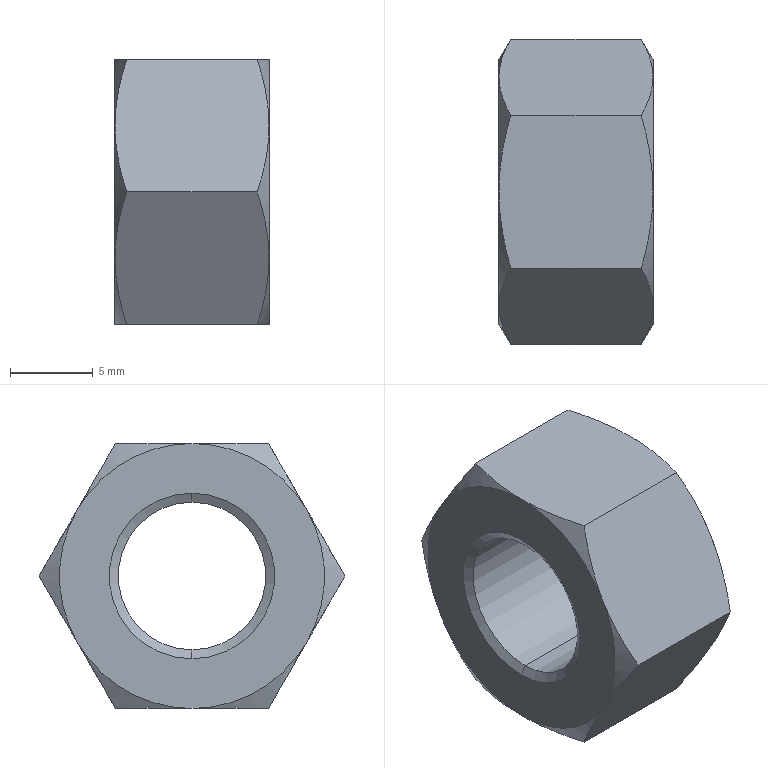Part | SolidWorks | features BaseBody 1 | 1 solid | 26 faces | box 9.3 x 18.475 x 16 mm | volume 1467 mm3 | cone 16 | plane 8 | cylinder 2 | commonest cylinder face diameters 8.917 x2
STEP:
#1=CARTESIAN_POINT('',(0.3125,0.,4.459));
#2=VERTEX_POINT('',#1);
#3=CARTESIAN_POINT('',(0.3125,0.,-4.459));
#4=VERTEX_POINT('',#3);
#5=CARTESIAN_POINT('',(0.3125,0.,0.));
#6=DIRECTION('',(1.,0.,0.));
#7=DIRECTION('',(0.,0.,-1.));
#8=AXIS2_PLACEMENT_3D('',#5,#6,#7);
#9=CIRCLE('',#8,4.459);
#10=EDGE_CURVE('',#2,#4,#9,.T.);
#11=ORIENTED_EDGE('',*,*,#10,.F.);
#12=CARTESIAN_POINT('',(8.987,0.,4.459));
#13=VERTEX_POINT('',#12);
#14=CARTESIAN_POINT('',(-16.85,0.,4.459));
#15=DIRECTION('',(1.,0.,0.));
#16=VECTOR('',#15,1000.);
#17=LINE('',#14,#16);
#18=EDGE_CURVE('',#2,#13,#17,.T.);
#19=ORIENTED_EDGE('',*,*,#18,.T.);
#20=CARTESIAN_POINT('',(8.987,0.,-4.459));
#21=VERTEX_POINT('',#20);
#22=CARTESIAN_POINT('',(8.987,0.,0.));
#23=DIRECTION('',(-1.,0.,0.));
#24=DIRECTION('',(0.,0.,-1.));
#25=AXIS2_PLACEMENT_3D('',#22,#23,#24);
#26=CIRCLE('',#25,4.459);
#27=EDGE_CURVE('',#21,#13,#26,.T.);
#28=ORIENTED_EDGE('',*,*,#27,.F.);
#29=CARTESIAN_POINT('',(-16.85,0.,-4.459));
#30=DIRECTION('',(1.,0.,0.));
#31=VECTOR('',#30,1000.);
#32=LINE('',#29,#31);
#33=EDGE_CURVE('',#4,#21,#32,.T.);
#34=ORIENTED_EDGE('',*,*,#33,.F.);
#35=EDGE_LOOP('',(#11,#19,#28,#34));
#36=FACE_OUTER_BOUND('',#35,.T.);
#37=CARTESIAN_POINT('',(-16.85,0.,0.));
#38=DIRECTION('',(1.,0.,0.));
#39=DIRECTION('',(0.,0.,-1.));
#40=AXIS2_PLACEMENT_3D('',#37,#38,#39);
#41=CYLINDRICAL_SURFACE('',#40,4.459);
#42=ADVANCED_FACE('',(#36),#41,.F.);
#43=ORIENTED_EDGE('',*,*,#10,.T.);
#44=CARTESIAN_POINT('',(0.,0.,-5.));
#45=VERTEX_POINT('',#44);
#46=CARTESIAN_POINT('',(0.,0.,-5.));
#47=DIRECTION('',(-0.5,0.,-0.866));
#48=VECTOR('',#47,1000.);
#49=LINE('',#46,#48);
#50=EDGE_CURVE('',#4,#45,#49,.T.);
#51=ORIENTED_EDGE('',*,*,#50,.T.);
#52=CARTESIAN_POINT('',(0.,0.,5.));
#53=VERTEX_POINT('',#52);
#54=CARTESIAN_POINT('',(0.,0.,0.));
#55=DIRECTION('',(1.,0.,0.));
#56=DIRECTION('',(0.,0.,1.));
#57=AXIS2_PLACEMENT_3D('',#54,#55,#56);
#58=CIRCLE('',#57,5.);
#59=EDGE_CURVE('',#53,#45,#58,.T.);
#60=ORIENTED_EDGE('',*,*,#59,.F.);
#61=CARTESIAN_POINT('',(0.,0.,5.));
#62=DIRECTION('',(-0.5,0.,0.866));
#63=VECTOR('',#62,1000.);
#64=LINE('',#61,#63);
#65=EDGE_CURVE('',#2,#53,#64,.T.);
#66=ORIENTED_EDGE('',*,*,#65,.F.);
#67=EDGE_LOOP('',(#43,#51,#60,#66));
#68=FACE_OUTER_BOUND('',#67,.T.);
#69=CARTESIAN_POINT('',(0.,0.,0.));
#70=DIRECTION('',(-1.,0.,0.));
#71=DIRECTION('',(0.,0.,1.));
#72=AXIS2_PLACEMENT_3D('',#69,#70,#71);
#73=CONICAL_SURFACE('',#72,5.,1.047);
#74=ADVANCED_FACE('',(#68),#73,.F.);
#75=ORIENTED_EDGE('',*,*,#27,.T.);
#76=CARTESIAN_POINT('',(9.3,0.,5.));
#77=VERTEX_POINT('',#76);
#78=CARTESIAN_POINT('',(9.3,0.,5.));
#79=DIRECTION('',(0.5,0.,0.866));
#80=VECTOR('',#79,1000.);
#81=LINE('',#78,#80);
#82=EDGE_CURVE('',#13,#77,#81,.T.);
#83=ORIENTED_EDGE('',*,*,#82,.T.);
#84=CARTESIAN_POINT('',(9.3,0.,-5.));
#85=VERTEX_POINT('',#84);
#86=CARTESIAN_POINT('',(9.3,0.,0.));
#87=DIRECTION('',(-1.,0.,0.));
#88=DIRECTION('',(0.,0.,-1.));
#89=AXIS2_PLACEMENT_3D('',#86,#87,#88);
#90=CIRCLE('',#89,5.);
#91=EDGE_CURVE('',#85,#77,#90,.T.);
#92=ORIENTED_EDGE('',*,*,#91,.F.);
#93=CARTESIAN_POINT('',(9.3,0.,-5.));
#94=DIRECTION('',(0.5,0.,-0.866));
#95=VECTOR('',#94,1000.);
#96=LINE('',#93,#95);
#97=EDGE_CURVE('',#21,#85,#96,.T.);
#98=ORIENTED_EDGE('',*,*,#97,.F.);
#99=EDGE_LOOP('',(#75,#83,#92,#98));
#100=FACE_OUTER_BOUND('',#99,.T.);
#101=CARTESIAN_POINT('',(9.3,0.,0.));
#102=DIRECTION('',(1.,0.,0.));
#103=DIRECTION('',(0.,0.,-1.));
#104=AXIS2_PLACEMENT_3D('',#101,#102,#103);
#105=CONICAL_SURFACE('',#104,5.,1.047);
#106=ADVANCED_FACE('',(#100),#105,.F.);
#107=ORIENTED_EDGE('',*,*,#18,.F.);
#108=CARTESIAN_POINT('',(0.3125,0.,0.));
#109=DIRECTION('',(1.,0.,0.));
#110=DIRECTION('',(0.,0.,-1.));
#111=AXIS2_PLACEMENT_3D('',#108,#109,#110);
#112=CIRCLE('',#111,4.459);
#113=EDGE_CURVE('',#4,#2,#112,.T.);
#114=ORIENTED_EDGE('',*,*,#113,.F.);
#115=ORIENTED_EDGE('',*,*,#33,.T.);
#116=CARTESIAN_POINT('',(8.987,0.,0.));
#117=DIRECTION('',(-1.,0.,0.));
#118=DIRECTION('',(0.,0.,-1.));
#119=AXIS2_PLACEMENT_3D('',#116,#117,#118);
#120=CIRCLE('',#119,4.459);
#121=EDGE_CURVE('',#13,#21,#120,.T.);
#122=ORIENTED_EDGE('',*,*,#121,.F.);
#123=EDGE_LOOP('',(#107,#114,#115,#122));
#124=FACE_OUTER_BOUND('',#123,.T.);
#125=CARTESIAN_POINT('',(-16.85,0.,0.));
#126=DIRECTION('',(1.,0.,0.));
#127=DIRECTION('',(0.,0.,-1.));
#128=AXIS2_PLACEMENT_3D('',#125,#126,#127);
#129=CYLINDRICAL_SURFACE('',#128,4.459);
#130=ADVANCED_FACE('',(#124),#129,.F.);
#131=ORIENTED_EDGE('',*,*,#50,.F.);
#132=ORIENTED_EDGE('',*,*,#113,.T.);
#133=ORIENTED_EDGE('',*,*,#65,.T.);
#134=CARTESIAN_POINT('',(0.,0.,0.));
#135=DIRECTION('',(1.,0.,0.));
#136=DIRECTION('',(0.,0.,1.));
#137=AXIS2_PLACEMENT_3D('',#134,#135,#136);
#138=CIRCLE('',#137,5.);
#139=EDGE_CURVE('',#45,#53,#138,.T.);
#140=ORIENTED_EDGE('',*,*,#139,.F.);
#141=EDGE_LOOP('',(#131,#132,#133,#140));
#142=FACE_OUTER_BOUND('',#141,.T.);
#143=CARTESIAN_POINT('',(0.,0.,0.));
#144=DIRECTION('',(-1.,0.,0.));
#145=DIRECTION('',(0.,0.,1.));
#146=AXIS2_PLACEMENT_3D('',#143,#144,#145);
#147=CONICAL_SURFACE('',#146,5.,1.047);
#148=ADVANCED_FACE('',(#142),#147,.F.);
#149=ORIENTED_EDGE('',*,*,#82,.F.);
#150=ORIENTED_EDGE('',*,*,#121,.T.);
#151=ORIENTED_EDGE('',*,*,#97,.T.);
#152=CARTESIAN_POINT('',(9.3,0.,0.));
#153=DIRECTION('',(-1.,0.,0.));
#154=DIRECTION('',(0.,0.,-1.));
#155=AXIS2_PLACEMENT_3D('',#152,#153,#154);
#156=CIRCLE('',#155,5.);
#157=EDGE_CURVE('',#77,#85,#156,.T.);
#158=ORIENTED_EDGE('',*,*,#157,.F.);
#159=EDGE_LOOP('',(#149,#150,#151,#158));
#160=FACE_OUTER_BOUND('',#159,.T.);
#161=CARTESIAN_POINT('',(9.3,0.,0.));
#162=DIRECTION('',(1.,0.,0.));
#163=DIRECTION('',(0.,0.,-1.));
#164=AXIS2_PLACEMENT_3D('',#161,#162,#163);
#165=CONICAL_SURFACE('',#164,5.,1.047);
#166=ADVANCED_FACE('',(#160),#165,.F.);
#167=ORIENTED_EDGE('',*,*,#59,.T.);
#168=ORIENTED_EDGE('',*,*,#139,.T.);
#169=EDGE_LOOP('',(#167,#168));
#170=FACE_BOUND('',#169,.T.);
#171=CARTESIAN_POINT('',(0.,0.,8.));
#172=VERTEX_POINT('',#171);
#173=CARTESIAN_POINT('',(0.,-6.928,4.));
#174=VERTEX_POINT('',#173);
#175=CARTESIAN_POINT('',(0.,0.,0.));
#176=DIRECTION('',(1.,0.,0.));
#177=DIRECTION('',(0.,0.,-1.));
#178=AXIS2_PLACEMENT_3D('',#175,#176,#177);
#179=CIRCLE('',#178,8.);
#180=EDGE_CURVE('',#172,#174,#179,.T.);
#181=ORIENTED_EDGE('',*,*,#180,.F.);
#182=CARTESIAN_POINT('',(0.,6.928,4.));
#183=VERTEX_POINT('',#182);
#184=CARTESIAN_POINT('',(0.,0.,0.));
#185=DIRECTION('',(1.,0.,0.));
#186=DIRECTION('',(0.,0.,-1.));
#187=AXIS2_PLACEMENT_3D('',#184,#185,#186);
#188=CIRCLE('',#187,8.);
#189=EDGE_CURVE('',#183,#172,#188,.T.);
#190=ORIENTED_EDGE('',*,*,#189,.F.);
#191=CARTESIAN_POINT('',(0.,6.928,-4.));
#192=VERTEX_POINT('',#191);
#193=CARTESIAN_POINT('',(0.,0.,0.));
#194=DIRECTION('',(1.,0.,0.));
#195=DIRECTION('',(0.,0.,-1.));
#196=AXIS2_PLACEMENT_3D('',#193,#194,#195);
#197=CIRCLE('',#196,8.);
#198=EDGE_CURVE('',#192,#183,#197,.T.);
#199=ORIENTED_EDGE('',*,*,#198,.F.);
#200=CARTESIAN_POINT('',(0.,0.,-8.));
#201=VERTEX_POINT('',#200);
#202=CARTESIAN_POINT('',(0.,0.,0.));
#203=DIRECTION('',(1.,0.,0.));
#204=DIRECTION('',(0.,0.,-1.));
#205=AXIS2_PLACEMENT_3D('',#202,#203,#204);
#206=CIRCLE('',#205,8.);
#207=EDGE_CURVE('',#201,#192,#206,.T.);
#208=ORIENTED_EDGE('',*,*,#207,.F.);
#209=CARTESIAN_POINT('',(0.,-6.928,-4.));
#210=VERTEX_POINT('',#209);
#211=CARTESIAN_POINT('',(0.,0.,0.));
#212=DIRECTION('',(1.,0.,0.));
#213=DIRECTION('',(0.,0.,-1.));
#214=AXIS2_PLACEMENT_3D('',#211,#212,#213);
#215=CIRCLE('',#214,8.);
#216=EDGE_CURVE('',#210,#201,#215,.T.);
#217=ORIENTED_EDGE('',*,*,#216,.F.);
#218=CARTESIAN_POINT('',(0.,0.,0.));
#219=DIRECTION('',(1.,0.,0.));
#220=DIRECTION('',(0.,0.,-1.));
#221=AXIS2_PLACEMENT_3D('',#218,#219,#220);
#222=CIRCLE('',#221,8.);
#223=EDGE_CURVE('',#174,#210,#222,.T.);
#224=ORIENTED_EDGE('',*,*,#223,.F.);
#225=EDGE_LOOP('',(#181,#190,#199,#208,#217,#224));
#226=FACE_OUTER_BOUND('',#225,.T.);
#227=CARTESIAN_POINT('',(0.,0.,0.));
#228=DIRECTION('',(1.,0.,0.));
#229=DIRECTION('',(0.,0.,-1.));
#230=AXIS2_PLACEMENT_3D('',#227,#228,#229);
#231=PLANE('',#230);
#232=ADVANCED_FACE('',(#170,#226),#231,.F.);
#233=ORIENTED_EDGE('',*,*,#91,.T.);
#234=ORIENTED_EDGE('',*,*,#157,.T.);
#235=EDGE_LOOP('',(#233,#234));
#236=FACE_BOUND('',#235,.T.);
#237=CARTESIAN_POINT('',(9.3,0.,8.));
#238=VERTEX_POINT('',#237);
#239=CARTESIAN_POINT('',(9.3,-6.928,4.));
#240=VERTEX_POINT('',#239);
#241=CARTESIAN_POINT('',(9.3,0.,0.));
#242=DIRECTION('',(1.,0.,0.));
#243=DIRECTION('',(0.,0.,1.));
#244=AXIS2_PLACEMENT_3D('',#241,#242,#243);
#245=CIRCLE('',#244,8.);
#246=EDGE_CURVE('',#238,#240,#245,.T.);
#247=ORIENTED_EDGE('',*,*,#246,.T.);
#248=CARTESIAN_POINT('',(9.3,-6.928,-4.));
#249=VERTEX_POINT('',#248);
#250=CARTESIAN_POINT('',(9.3,0.,0.));
#251=DIRECTION('',(1.,0.,0.));
#252=DIRECTION('',(0.,0.,1.));
#253=AXIS2_PLACEMENT_3D('',#250,#251,#252);
#254=CIRCLE('',#253,8.);
#255=EDGE_CURVE('',#240,#249,#254,.T.);
#256=ORIENTED_EDGE('',*,*,#255,.T.);
#257=CARTESIAN_POINT('',(9.3,0.,-8.));
#258=VERTEX_POINT('',#257);
#259=CARTESIAN_POINT('',(9.3,0.,0.));
#260=DIRECTION('',(1.,0.,0.));
#261=DIRECTION('',(0.,0.,1.));
#262=AXIS2_PLACEMENT_3D('',#259,#260,#261);
#263=CIRCLE('',#262,8.);
#264=EDGE_CURVE('',#249,#258,#263,.T.);
#265=ORIENTED_EDGE('',*,*,#264,.T.);
#266=CARTESIAN_POINT('',(9.3,6.928,-4.));
#267=VERTEX_POINT('',#266);
#268=CARTESIAN_POINT('',(9.3,0.,0.));
#269=DIRECTION('',(1.,0.,0.));
#270=DIRECTION('',(0.,0.,1.));
#271=AXIS2_PLACEMENT_3D('',#268,#269,#270);
#272=CIRCLE('',#271,8.);
#273=EDGE_CURVE('',#258,#267,#272,.T.);
#274=ORIENTED_EDGE('',*,*,#273,.T.);
#275=CARTESIAN_POINT('',(9.3,6.928,4.));
#276=VERTEX_POINT('',#275);
#277=CARTESIAN_POINT('',(9.3,0.,0.));
#278=DIRECTION('',(1.,0.,0.));
#279=DIRECTION('',(0.,0.,1.));
#280=AXIS2_PLACEMENT_3D('',#277,#278,#279);
#281=CIRCLE('',#280,8.);
#282=EDGE_CURVE('',#267,#276,#281,.T.);
#283=ORIENTED_EDGE('',*,*,#282,.T.);
#284=CARTESIAN_POINT('',(9.3,0.,0.));
#285=DIRECTION('',(1.,0.,0.));
#286=DIRECTION('',(0.,0.,1.));
#287=AXIS2_PLACEMENT_3D('',#284,#285,#286);
#288=CIRCLE('',#287,8.);
#289=EDGE_CURVE('',#276,#238,#288,.T.);
#290=ORIENTED_EDGE('',*,*,#289,.T.);
#291=EDGE_LOOP('',(#247,#256,#265,#274,#283,#290));
#292=FACE_OUTER_BOUND('',#291,.T.);
#293=CARTESIAN_POINT('',(9.3,0.,0.));
#294=DIRECTION('',(1.,0.,0.));
#295=DIRECTION('',(0.,0.,-1.));
#296=AXIS2_PLACEMENT_3D('',#293,#294,#295);
#297=PLANE('',#296);
#298=ADVANCED_FACE('',(#236,#292),#297,.T.);
#299=ORIENTED_EDGE('',*,*,#223,.T.);
#300=CARTESIAN_POINT('',(0.7145,-9.238,0.000000014));
#301=VERTEX_POINT('',#300);
#302=CARTESIAN_POINT('',(0.,-6.928,-4.));
#303=CARTESIAN_POINT('',(0.,-7.322,-3.317));
#304=CARTESIAN_POINT('',(0.06831,-7.711,-2.644));
#305=CARTESIAN_POINT('',(0.3171,-8.48,-1.312));
#306=CARTESIAN_POINT('',(0.4967,-8.86,-0.6534));
#307=CARTESIAN_POINT('',(0.7145,-9.238,0.000000014));
#308=B_SPLINE_CURVE_WITH_KNOTS('',3,(#302,#303,#304,#305,#306,#307),.UNSPECIFIED.,.F.,.F.,(4,2,4),(0.,0.002337,0.004674),.UNSPECIFIED.);
#309=EDGE_CURVE('',#210,#301,#308,.T.);
#310=ORIENTED_EDGE('',*,*,#309,.T.);
#311=CARTESIAN_POINT('',(0.7145,-9.238,0.000000014));
#312=CARTESIAN_POINT('',(0.4967,-8.86,0.6534));
#313=CARTESIAN_POINT('',(0.3171,-8.48,1.312));
#314=CARTESIAN_POINT('',(0.06831,-7.711,2.644));
#315=CARTESIAN_POINT('',(0.,-7.322,3.317));
#316=CARTESIAN_POINT('',(0.,-6.928,4.));
#317=B_SPLINE_CURVE_WITH_KNOTS('',3,(#311,#312,#313,#314,#315,#316),.UNSPECIFIED.,.F.,.F.,(4,2,4),(0.,0.002337,0.004674),.UNSPECIFIED.);
#318=EDGE_CURVE('',#301,#174,#317,.T.);
#319=ORIENTED_EDGE('',*,*,#318,.T.);
#320=EDGE_LOOP('',(#299,#310,#319));
#321=FACE_OUTER_BOUND('',#320,.T.);
#322=CARTESIAN_POINT('',(0.7188,0.,0.));
#323=DIRECTION('',(1.,0.,0.));
#324=DIRECTION('',(0.,0.,-1.));
#325=AXIS2_PLACEMENT_3D('',#322,#323,#324);
#326=CONICAL_SURFACE('',#325,9.245,1.047);
#327=ADVANCED_FACE('',(#321),#326,.T.);
#328=ORIENTED_EDGE('',*,*,#180,.T.);
#329=CARTESIAN_POINT('',(0.7145,-4.619,8.));
#330=VERTEX_POINT('',#329);
#331=CARTESIAN_POINT('',(0.,-6.928,4.));
#332=CARTESIAN_POINT('',(0.,-6.534,4.683));
#333=CARTESIAN_POINT('',(0.06831,-6.145,5.356));
#334=CARTESIAN_POINT('',(0.3171,-5.376,6.688));
#335=CARTESIAN_POINT('',(0.4967,-4.996,7.347));
#336=CARTESIAN_POINT('',(0.7145,-4.619,8.));
#337=B_SPLINE_CURVE_WITH_KNOTS('',3,(#331,#332,#333,#334,#335,#336),.UNSPECIFIED.,.F.,.F.,(4,2,4),(0.,0.002337,0.004674),.UNSPECIFIED.);
#338=EDGE_CURVE('',#174,#330,#337,.T.);
#339=ORIENTED_EDGE('',*,*,#338,.T.);
#340=CARTESIAN_POINT('',(0.7145,-4.619,8.));
#341=CARTESIAN_POINT('',(0.4967,-3.864,8.));
#342=CARTESIAN_POINT('',(0.3171,-3.104,8.));
#343=CARTESIAN_POINT('',(0.06831,-1.566,8.));
#344=CARTESIAN_POINT('',(0.,-0.7882,8.));
#345=CARTESIAN_POINT('',(0.,0.,8.));
#346=B_SPLINE_CURVE_WITH_KNOTS('',3,(#340,#341,#342,#343,#344,#345),.UNSPECIFIED.,.F.,.F.,(4,2,4),(0.,0.002337,0.004674),.UNSPECIFIED.);
#347=EDGE_CURVE('',#330,#172,#346,.T.);
#348=ORIENTED_EDGE('',*,*,#347,.T.);
#349=EDGE_LOOP('',(#328,#339,#348));
#350=FACE_OUTER_BOUND('',#349,.T.);
#351=CARTESIAN_POINT('',(0.7188,0.,0.));
#352=DIRECTION('',(1.,0.,0.));
#353=DIRECTION('',(0.,0.,-1.));
#354=AXIS2_PLACEMENT_3D('',#351,#352,#353);
#355=CONICAL_SURFACE('',#354,9.245,1.047);
#356=ADVANCED_FACE('',(#350),#355,.T.);
#357=ORIENTED_EDGE('',*,*,#189,.T.);
#358=CARTESIAN_POINT('',(0.7145,4.619,8.));
#359=VERTEX_POINT('',#358);
#360=CARTESIAN_POINT('',(0.,0.,8.));
#361=CARTESIAN_POINT('',(0.,0.7882,8.));
#362=CARTESIAN_POINT('',(0.06831,1.566,8.));
#363=CARTESIAN_POINT('',(0.3171,3.104,8.));
#364=CARTESIAN_POINT('',(0.4967,3.864,8.));
#365=CARTESIAN_POINT('',(0.7145,4.619,8.));
#366=B_SPLINE_CURVE_WITH_KNOTS('',3,(#360,#361,#362,#363,#364,#365),.UNSPECIFIED.,.F.,.F.,(4,2,4),(0.,0.002337,0.004674),.UNSPECIFIED.);
#367=EDGE_CURVE('',#172,#359,#366,.T.);
#368=ORIENTED_EDGE('',*,*,#367,.T.);
#369=CARTESIAN_POINT('',(0.7145,4.619,8.));
#370=CARTESIAN_POINT('',(0.4967,4.996,7.347));
#371=CARTESIAN_POINT('',(0.3171,5.376,6.688));
#372=CARTESIAN_POINT('',(0.06831,6.145,5.356));
#373=CARTESIAN_POINT('',(0.,6.534,4.683));
#374=CARTESIAN_POINT('',(0.,6.928,4.));
#375=B_SPLINE_CURVE_WITH_KNOTS('',3,(#369,#370,#371,#372,#373,#374),.UNSPECIFIED.,.F.,.F.,(4,2,4),(0.,0.002337,0.004674),.UNSPECIFIED.);
#376=EDGE_CURVE('',#359,#183,#375,.T.);
#377=ORIENTED_EDGE('',*,*,#376,.T.);
#378=EDGE_LOOP('',(#357,#368,#377));
#379=FACE_OUTER_BOUND('',#378,.T.);
#380=CARTESIAN_POINT('',(0.7188,0.,0.));
#381=DIRECTION('',(1.,0.,0.));
#382=DIRECTION('',(0.,0.,-1.));
#383=AXIS2_PLACEMENT_3D('',#380,#381,#382);
#384=CONICAL_SURFACE('',#383,9.245,1.047);
#385=ADVANCED_FACE('',(#379),#384,.T.);
#386=ORIENTED_EDGE('',*,*,#198,.T.);
#387=CARTESIAN_POINT('',(0.7145,9.238,-0.000000014));
#388=VERTEX_POINT('',#387);
#389=CARTESIAN_POINT('',(0.,6.928,4.));
#390=CARTESIAN_POINT('',(0.,7.322,3.317));
#391=CARTESIAN_POINT('',(0.06831,7.711,2.644));
#392=CARTESIAN_POINT('',(0.3171,8.48,1.312));
#393=CARTESIAN_POINT('',(0.4967,8.86,0.6534));
#394=CARTESIAN_POINT('',(0.7145,9.238,-0.000000014));
#395=B_SPLINE_CURVE_WITH_KNOTS('',3,(#389,#390,#391,#392,#393,#394),.UNSPECIFIED.,.F.,.F.,(4,2,4),(0.,0.002337,0.004674),.UNSPECIFIED.);
#396=EDGE_CURVE('',#183,#388,#395,.T.);
#397=ORIENTED_EDGE('',*,*,#396,.T.);
#398=CARTESIAN_POINT('',(0.7145,9.238,-0.000000014));
#399=CARTESIAN_POINT('',(0.4967,8.86,-0.6534));
#400=CARTESIAN_POINT('',(0.3171,8.48,-1.312));
#401=CARTESIAN_POINT('',(0.06831,7.711,-2.644));
#402=CARTESIAN_POINT('',(0.,7.322,-3.317));
#403=CARTESIAN_POINT('',(0.,6.928,-4.));
#404=B_SPLINE_CURVE_WITH_KNOTS('',3,(#398,#399,#400,#401,#402,#403),.UNSPECIFIED.,.F.,.F.,(4,2,4),(0.,0.002337,0.004674),.UNSPECIFIED.);
#405=EDGE_CURVE('',#388,#192,#404,.T.);
#406=ORIENTED_EDGE('',*,*,#405,.T.);
#407=EDGE_LOOP('',(#386,#397,#406));
#408=FACE_OUTER_BOUND('',#407,.T.);
#409=CARTESIAN_POINT('',(0.7188,0.,0.));
#410=DIRECTION('',(1.,0.,0.));
#411=DIRECTION('',(0.,0.,-1.));
#412=AXIS2_PLACEMENT_3D('',#409,#410,#411);
#413=CONICAL_SURFACE('',#412,9.245,1.047);
#414=ADVANCED_FACE('',(#408),#413,.T.);
#415=CARTESIAN_POINT('',(0.7145,4.619,-8.));
#416=VERTEX_POINT('',#415);
#417=CARTESIAN_POINT('',(0.7145,4.619,-8.));
#418=CARTESIAN_POINT('',(0.4967,3.864,-8.));
#419=CARTESIAN_POINT('',(0.3171,3.104,-8.));
#420=CARTESIAN_POINT('',(0.06831,1.566,-8.));
#421=CARTESIAN_POINT('',(0.,0.7882,-8.));
#422=CARTESIAN_POINT('',(0.,0.,-8.));
#423=B_SPLINE_CURVE_WITH_KNOTS('',3,(#417,#418,#419,#420,#421,#422),.UNSPECIFIED.,.F.,.F.,(4,2,4),(0.,0.002337,0.004674),.UNSPECIFIED.);
#424=EDGE_CURVE('',#416,#201,#423,.T.);
#425=ORIENTED_EDGE('',*,*,#424,.T.);
#426=ORIENTED_EDGE('',*,*,#207,.T.);
#427=CARTESIAN_POINT('',(0.,6.928,-4.));
#428=CARTESIAN_POINT('',(0.,6.534,-4.683));
#429=CARTESIAN_POINT('',(0.06831,6.145,-5.356));
#430=CARTESIAN_POINT('',(0.3171,5.376,-6.688));
#431=CARTESIAN_POINT('',(0.4967,4.996,-7.347));
#432=CARTESIAN_POINT('',(0.7145,4.619,-8.));
#433=B_SPLINE_CURVE_WITH_KNOTS('',3,(#427,#428,#429,#430,#431,#432),.UNSPECIFIED.,.F.,.F.,(4,2,4),(0.,0.002337,0.004674),.UNSPECIFIED.);
#434=EDGE_CURVE('',#192,#416,#433,.T.);
#435=ORIENTED_EDGE('',*,*,#434,.T.);
#436=EDGE_LOOP('',(#425,#426,#435));
#437=FACE_OUTER_BOUND('',#436,.T.);
#438=CARTESIAN_POINT('',(0.7188,0.,0.));
#439=DIRECTION('',(1.,0.,0.));
#440=DIRECTION('',(0.,0.,-1.));
#441=AXIS2_PLACEMENT_3D('',#438,#439,#440);
#442=CONICAL_SURFACE('',#441,9.245,1.047);
#443=ADVANCED_FACE('',(#437),#442,.T.);
#444=CARTESIAN_POINT('',(0.7145,-4.619,-8.));
#445=VERTEX_POINT('',#444);
#446=CARTESIAN_POINT('',(0.7145,-4.619,-8.));
#447=CARTESIAN_POINT('',(0.4967,-4.996,-7.347));
#448=CARTESIAN_POINT('',(0.3171,-5.376,-6.688));
#449=CARTESIAN_POINT('',(0.06831,-6.145,-5.356));
#450=CARTESIAN_POINT('',(0.,-6.534,-4.683));
#451=CARTESIAN_POINT('',(0.,-6.928,-4.));
#452=B_SPLINE_CURVE_WITH_KNOTS('',3,(#446,#447,#448,#449,#450,#451),.UNSPECIFIED.,.F.,.F.,(4,2,4),(0.,0.002337,0.004674),.UNSPECIFIED.);
#453=EDGE_CURVE('',#445,#210,#452,.T.);
#454=ORIENTED_EDGE('',*,*,#453,.T.);
#455=ORIENTED_EDGE('',*,*,#216,.T.);
#456=CARTESIAN_POINT('',(0.,0.,-8.));
#457=CARTESIAN_POINT('',(0.,-0.7882,-8.));
#458=CARTESIAN_POINT('',(0.06831,-1.566,-8.));
#459=CARTESIAN_POINT('',(0.3171,-3.104,-8.));
#460=CARTESIAN_POINT('',(0.4967,-3.864,-8.));
#461=CARTESIAN_POINT('',(0.7145,-4.619,-8.));
#462=B_SPLINE_CURVE_WITH_KNOTS('',3,(#456,#457,#458,#459,#460,#461),.UNSPECIFIED.,.F.,.F.,(4,2,4),(0.,0.002337,0.004674),.UNSPECIFIED.);
#463=EDGE_CURVE('',#201,#445,#462,.T.);
#464=ORIENTED_EDGE('',*,*,#463,.T.);
#465=EDGE_LOOP('',(#454,#455,#464));
#466=FACE_OUTER_BOUND('',#465,.T.);
#467=CARTESIAN_POINT('',(0.7188,0.,0.));
#468=DIRECTION('',(1.,0.,0.));
#469=DIRECTION('',(0.,0.,-1.));
#470=AXIS2_PLACEMENT_3D('',#467,#468,#469);
#471=CONICAL_SURFACE('',#470,9.245,1.047);
#472=ADVANCED_FACE('',(#466),#471,.T.);
#473=CARTESIAN_POINT('',(8.585,-9.238,0.000000038));
#474=VERTEX_POINT('',#473);
#475=CARTESIAN_POINT('',(8.585,-9.238,0.000000038));
#476=CARTESIAN_POINT('',(8.803,-8.86,-0.6534));
#477=CARTESIAN_POINT('',(8.983,-8.48,-1.312));
#478=CARTESIAN_POINT('',(9.232,-7.711,-2.644));
#479=CARTESIAN_POINT('',(9.3,-7.322,-3.317));
#480=CARTESIAN_POINT('',(9.3,-6.928,-4.));
#481=B_SPLINE_CURVE_WITH_KNOTS('',3,(#475,#476,#477,#478,#479,#480),.UNSPECIFIED.,.F.,.F.,(4,2,4),(0.,0.002337,0.004674),.UNSPECIFIED.);
#482=EDGE_CURVE('',#474,#249,#481,.T.);
#483=ORIENTED_EDGE('',*,*,#482,.T.);
#484=ORIENTED_EDGE('',*,*,#255,.F.);
#485=CARTESIAN_POINT('',(9.3,-6.928,4.));
#486=CARTESIAN_POINT('',(9.3,-7.322,3.317));
#487=CARTESIAN_POINT('',(9.232,-7.711,2.644));
#488=CARTESIAN_POINT('',(8.983,-8.48,1.312));
#489=CARTESIAN_POINT('',(8.803,-8.86,0.6534));
#490=CARTESIAN_POINT('',(8.585,-9.238,0.000000038));
#491=B_SPLINE_CURVE_WITH_KNOTS('',3,(#485,#486,#487,#488,#489,#490),.UNSPECIFIED.,.F.,.F.,(4,2,4),(0.,0.002337,0.004674),.UNSPECIFIED.);
#492=EDGE_CURVE('',#240,#474,#491,.T.);
#493=ORIENTED_EDGE('',*,*,#492,.T.);
#494=EDGE_LOOP('',(#483,#484,#493));
#495=FACE_OUTER_BOUND('',#494,.T.);
#496=CARTESIAN_POINT('',(8.581,0.,0.));
#497=DIRECTION('',(-1.,0.,0.));
#498=DIRECTION('',(0.,0.,1.));
#499=AXIS2_PLACEMENT_3D('',#496,#497,#498);
#500=CONICAL_SURFACE('',#499,9.245,1.047);
#501=ADVANCED_FACE('',(#495),#500,.T.);
#502=CARTESIAN_POINT('',(8.585,-4.619,8.));
#503=VERTEX_POINT('',#502);
#504=CARTESIAN_POINT('',(8.585,-4.619,8.));
#505=CARTESIAN_POINT('',(8.803,-4.996,7.347));
#506=CARTESIAN_POINT('',(8.983,-5.376,6.688));
#507=CARTESIAN_POINT('',(9.232,-6.145,5.356));
#508=CARTESIAN_POINT('',(9.3,-6.534,4.683));
#509=CARTESIAN_POINT('',(9.3,-6.928,4.));
#510=B_SPLINE_CURVE_WITH_KNOTS('',3,(#504,#505,#506,#507,#508,#509),.UNSPECIFIED.,.F.,.F.,(4,2,4),(0.,0.002337,0.004674),.UNSPECIFIED.);
#511=EDGE_CURVE('',#503,#240,#510,.T.);
#512=ORIENTED_EDGE('',*,*,#511,.T.);
#513=ORIENTED_EDGE('',*,*,#246,.F.);
#514=CARTESIAN_POINT('',(9.3,0.,8.));
#515=CARTESIAN_POINT('',(9.3,-0.7882,8.));
#516=CARTESIAN_POINT('',(9.232,-1.566,8.));
#517=CARTESIAN_POINT('',(8.983,-3.104,8.));
#518=CARTESIAN_POINT('',(8.803,-3.864,8.));
#519=CARTESIAN_POINT('',(8.585,-4.619,8.));
#520=B_SPLINE_CURVE_WITH_KNOTS('',3,(#514,#515,#516,#517,#518,#519),.UNSPECIFIED.,.F.,.F.,(4,2,4),(0.,0.002337,0.004674),.UNSPECIFIED.);
#521=EDGE_CURVE('',#238,#503,#520,.T.);
#522=ORIENTED_EDGE('',*,*,#521,.T.);
#523=EDGE_LOOP('',(#512,#513,#522));
#524=FACE_OUTER_BOUND('',#523,.T.);
#525=CARTESIAN_POINT('',(8.581,0.,0.));
#526=DIRECTION('',(-1.,0.,0.));
#527=DIRECTION('',(0.,0.,1.));
#528=AXIS2_PLACEMENT_3D('',#525,#526,#527);
#529=CONICAL_SURFACE('',#528,9.245,1.047);
#530=ADVANCED_FACE('',(#524),#529,.T.);
#531=CARTESIAN_POINT('',(8.585,4.619,8.));
#532=VERTEX_POINT('',#531);
#533=CARTESIAN_POINT('',(8.585,4.619,8.));
#534=CARTESIAN_POINT('',(8.803,3.864,8.));
#535=CARTESIAN_POINT('',(8.983,3.104,8.));
#536=CARTESIAN_POINT('',(9.232,1.566,8.));
#537=CARTESIAN_POINT('',(9.3,0.7882,8.));
#538=CARTESIAN_POINT('',(9.3,0.,8.));
#539=B_SPLINE_CURVE_WITH_KNOTS('',3,(#533,#534,#535,#536,#537,#538),.UNSPECIFIED.,.F.,.F.,(4,2,4),(0.,0.002337,0.004674),.UNSPECIFIED.);
#540=EDGE_CURVE('',#532,#238,#539,.T.);
#541=ORIENTED_EDGE('',*,*,#540,.T.);
#542=ORIENTED_EDGE('',*,*,#289,.F.);
#543=CARTESIAN_POINT('',(9.3,6.928,4.));
#544=CARTESIAN_POINT('',(9.3,6.534,4.683));
#545=CARTESIAN_POINT('',(9.232,6.145,5.356));
#546=CARTESIAN_POINT('',(8.983,5.376,6.688));
#547=CARTESIAN_POINT('',(8.803,4.996,7.347));
#548=CARTESIAN_POINT('',(8.585,4.619,8.));
#549=B_SPLINE_CURVE_WITH_KNOTS('',3,(#543,#544,#545,#546,#547,#548),.UNSPECIFIED.,.F.,.F.,(4,2,4),(0.,0.002337,0.004674),.UNSPECIFIED.);
#550=EDGE_CURVE('',#276,#532,#549,.T.);
#551=ORIENTED_EDGE('',*,*,#550,.T.);
#552=EDGE_LOOP('',(#541,#542,#551));
#553=FACE_OUTER_BOUND('',#552,.T.);
#554=CARTESIAN_POINT('',(8.581,0.,0.));
#555=DIRECTION('',(-1.,0.,0.));
#556=DIRECTION('',(0.,0.,1.));
#557=AXIS2_PLACEMENT_3D('',#554,#555,#556);
#558=CONICAL_SURFACE('',#557,9.245,1.047);
#559=ADVANCED_FACE('',(#553),#558,.T.);
#560=ORIENTED_EDGE('',*,*,#282,.F.);
#561=CARTESIAN_POINT('',(8.585,9.238,0.000000014));
#562=VERTEX_POINT('',#561);
#563=CARTESIAN_POINT('',(9.3,6.928,-4.));
#564=CARTESIAN_POINT('',(9.3,7.322,-3.317));
#565=CARTESIAN_POINT('',(9.232,7.711,-2.644));
#566=CARTESIAN_POINT('',(8.983,8.48,-1.312));
#567=CARTESIAN_POINT('',(8.803,8.86,-0.6534));
#568=CARTESIAN_POINT('',(8.585,9.238,0.000000014));
#569=B_SPLINE_CURVE_WITH_KNOTS('',3,(#563,#564,#565,#566,#567,#568),.UNSPECIFIED.,.F.,.F.,(4,2,4),(0.,0.002337,0.004674),.UNSPECIFIED.);
#570=EDGE_CURVE('',#267,#562,#569,.T.);
#571=ORIENTED_EDGE('',*,*,#570,.T.);
#572=CARTESIAN_POINT('',(8.585,9.238,0.000000014));
#573=CARTESIAN_POINT('',(8.803,8.86,0.6534));
#574=CARTESIAN_POINT('',(8.983,8.48,1.312));
#575=CARTESIAN_POINT('',(9.232,7.711,2.644));
#576=CARTESIAN_POINT('',(9.3,7.322,3.317));
#577=CARTESIAN_POINT('',(9.3,6.928,4.));
#578=B_SPLINE_CURVE_WITH_KNOTS('',3,(#572,#573,#574,#575,#576,#577),.UNSPECIFIED.,.F.,.F.,(4,2,4),(0.,0.002337,0.004674),.UNSPECIFIED.);
#579=EDGE_CURVE('',#562,#276,#578,.T.);
#580=ORIENTED_EDGE('',*,*,#579,.T.);
#581=EDGE_LOOP('',(#560,#571,#580));
#582=FACE_OUTER_BOUND('',#581,.T.);
#583=CARTESIAN_POINT('',(8.581,0.,0.));
#584=DIRECTION('',(-1.,0.,0.));
#585=DIRECTION('',(0.,0.,1.));
#586=AXIS2_PLACEMENT_3D('',#583,#584,#585);
#587=CONICAL_SURFACE('',#586,9.245,1.047);
#588=ADVANCED_FACE('',(#582),#587,.T.);
#589=ORIENTED_EDGE('',*,*,#273,.F.);
#590=CARTESIAN_POINT('',(8.585,4.619,-8.));
#591=VERTEX_POINT('',#590);
#592=CARTESIAN_POINT('',(9.3,0.,-8.));
#593=CARTESIAN_POINT('',(9.3,0.7882,-8.));
#594=CARTESIAN_POINT('',(9.232,1.566,-8.));
#595=CARTESIAN_POINT('',(8.983,3.104,-8.));
#596=CARTESIAN_POINT('',(8.803,3.864,-8.));
#597=CARTESIAN_POINT('',(8.585,4.619,-8.));
#598=B_SPLINE_CURVE_WITH_KNOTS('',3,(#592,#593,#594,#595,#596,#597),.UNSPECIFIED.,.F.,.F.,(4,2,4),(0.,0.002337,0.004674),.UNSPECIFIED.);
#599=EDGE_CURVE('',#258,#591,#598,.T.);
#600=ORIENTED_EDGE('',*,*,#599,.T.);
#601=CARTESIAN_POINT('',(8.585,4.619,-8.));
#602=CARTESIAN_POINT('',(8.803,4.996,-7.347));
#603=CARTESIAN_POINT('',(8.983,5.376,-6.688));
#604=CARTESIAN_POINT('',(9.232,6.145,-5.356));
#605=CARTESIAN_POINT('',(9.3,6.534,-4.683));
#606=CARTESIAN_POINT('',(9.3,6.928,-4.));
#607=B_SPLINE_CURVE_WITH_KNOTS('',3,(#601,#602,#603,#604,#605,#606),.UNSPECIFIED.,.F.,.F.,(4,2,4),(0.,0.002337,0.004674),.UNSPECIFIED.);
#608=EDGE_CURVE('',#591,#267,#607,.T.);
#609=ORIENTED_EDGE('',*,*,#608,.T.);
#610=EDGE_LOOP('',(#589,#600,#609));
#611=FACE_OUTER_BOUND('',#610,.T.);
#612=CARTESIAN_POINT('',(8.581,0.,0.));
#613=DIRECTION('',(-1.,0.,0.));
#614=DIRECTION('',(0.,0.,1.));
#615=AXIS2_PLACEMENT_3D('',#612,#613,#614);
#616=CONICAL_SURFACE('',#615,9.245,1.047);
#617=ADVANCED_FACE('',(#611),#616,.T.);
#618=ORIENTED_EDGE('',*,*,#264,.F.);
#619=CARTESIAN_POINT('',(8.585,-4.619,-8.));
#620=VERTEX_POINT('',#619);
#621=CARTESIAN_POINT('',(9.3,-6.928,-4.));
#622=CARTESIAN_POINT('',(9.3,-6.534,-4.683));
#623=CARTESIAN_POINT('',(9.232,-6.145,-5.356));
#624=CARTESIAN_POINT('',(8.983,-5.376,-6.688));
#625=CARTESIAN_POINT('',(8.803,-4.996,-7.347));
#626=CARTESIAN_POINT('',(8.585,-4.619,-8.));
#627=B_SPLINE_CURVE_WITH_KNOTS('',3,(#621,#622,#623,#624,#625,#626),.UNSPECIFIED.,.F.,.F.,(4,2,4),(0.,0.002337,0.004674),.UNSPECIFIED.);
#628=EDGE_CURVE('',#249,#620,#627,.T.);
#629=ORIENTED_EDGE('',*,*,#628,.T.);
#630=CARTESIAN_POINT('',(8.585,-4.619,-8.));
#631=CARTESIAN_POINT('',(8.803,-3.864,-8.));
#632=CARTESIAN_POINT('',(8.983,-3.104,-8.));
#633=CARTESIAN_POINT('',(9.232,-1.566,-8.));
#634=CARTESIAN_POINT('',(9.3,-0.7882,-8.));
#635=CARTESIAN_POINT('',(9.3,0.,-8.));
#636=B_SPLINE_CURVE_WITH_KNOTS('',3,(#630,#631,#632,#633,#634,#635),.UNSPECIFIED.,.F.,.F.,(4,2,4),(0.,0.002337,0.004674),.UNSPECIFIED.);
#637=EDGE_CURVE('',#620,#258,#636,.T.);
#638=ORIENTED_EDGE('',*,*,#637,.T.);
#639=EDGE_LOOP('',(#618,#629,#638));
#640=FACE_OUTER_BOUND('',#639,.T.);
#641=CARTESIAN_POINT('',(8.581,0.,0.));
#642=DIRECTION('',(-1.,0.,0.));
#643=DIRECTION('',(0.,0.,1.));
#644=AXIS2_PLACEMENT_3D('',#641,#642,#643);
#645=CONICAL_SURFACE('',#644,9.245,1.047);
#646=ADVANCED_FACE('',(#640),#645,.T.);
#647=CARTESIAN_POINT('',(0.,-9.238,0.));
#648=DIRECTION('',(-1.,0.,0.));
#649=VECTOR('',#648,1000.);
#650=LINE('',#647,#649);
#651=EDGE_CURVE('',#474,#301,#650,.T.);
#652=ORIENTED_EDGE('',*,*,#651,.T.);
#653=ORIENTED_EDGE('',*,*,#309,.F.);
#654=ORIENTED_EDGE('',*,*,#453,.F.);
#655=CARTESIAN_POINT('',(0.,-4.619,-8.));
#656=DIRECTION('',(1.,0.,0.));
#657=VECTOR('',#656,1000.);
#658=LINE('',#655,#657);
#659=EDGE_CURVE('',#445,#620,#658,.T.);
#660=ORIENTED_EDGE('',*,*,#659,.T.);
#661=ORIENTED_EDGE('',*,*,#628,.F.);
#662=ORIENTED_EDGE('',*,*,#482,.F.);
#663=EDGE_LOOP('',(#652,#653,#654,#660,#661,#662));
#664=FACE_OUTER_BOUND('',#663,.T.);
#665=CARTESIAN_POINT('',(0.,-4.619,-8.));
#666=DIRECTION('',(0.,-0.866,-0.5));
#667=DIRECTION('',(0.,0.5,-0.866));
#668=AXIS2_PLACEMENT_3D('',#665,#666,#667);
#669=PLANE('',#668);
#670=ADVANCED_FACE('',(#664),#669,.T.);
#671=ORIENTED_EDGE('',*,*,#511,.F.);
#672=CARTESIAN_POINT('',(0.,-4.619,8.));
#673=DIRECTION('',(-1.,0.,0.));
#674=VECTOR('',#673,1000.);
#675=LINE('',#672,#674);
#676=EDGE_CURVE('',#503,#330,#675,.T.);
#677=ORIENTED_EDGE('',*,*,#676,.T.);
#678=ORIENTED_EDGE('',*,*,#338,.F.);
#679=ORIENTED_EDGE('',*,*,#318,.F.);
#680=ORIENTED_EDGE('',*,*,#651,.F.);
#681=ORIENTED_EDGE('',*,*,#492,.F.);
#682=EDGE_LOOP('',(#671,#677,#678,#679,#680,#681));
#683=FACE_OUTER_BOUND('',#682,.T.);
#684=CARTESIAN_POINT('',(0.,-9.238,0.));
#685=DIRECTION('',(0.,-0.866,0.5));
#686=DIRECTION('',(0.,-0.5,-0.866));
#687=AXIS2_PLACEMENT_3D('',#684,#685,#686);
#688=PLANE('',#687);
#689=ADVANCED_FACE('',(#683),#688,.T.);
#690=ORIENTED_EDGE('',*,*,#540,.F.);
#691=CARTESIAN_POINT('',(0.,4.619,8.));
#692=DIRECTION('',(-1.,0.,0.));
#693=VECTOR('',#692,1000.);
#694=LINE('',#691,#693);
#695=EDGE_CURVE('',#532,#359,#694,.T.);
#696=ORIENTED_EDGE('',*,*,#695,.T.);
#697=ORIENTED_EDGE('',*,*,#367,.F.);
#698=ORIENTED_EDGE('',*,*,#347,.F.);
#699=ORIENTED_EDGE('',*,*,#676,.F.);
#700=ORIENTED_EDGE('',*,*,#521,.F.);
#701=EDGE_LOOP('',(#690,#696,#697,#698,#699,#700));
#702=FACE_OUTER_BOUND('',#701,.T.);
#703=CARTESIAN_POINT('',(0.,-4.619,8.));
#704=DIRECTION('',(0.,0.,1.));
#705=DIRECTION('',(1.,0.,0.));
#706=AXIS2_PLACEMENT_3D('',#703,#704,#705);
#707=PLANE('',#706);
#708=ADVANCED_FACE('',(#702),#707,.T.);
#709=ORIENTED_EDGE('',*,*,#579,.F.);
#710=CARTESIAN_POINT('',(0.,9.238,0.));
#711=DIRECTION('',(-1.,0.,0.));
#712=VECTOR('',#711,1000.);
#713=LINE('',#710,#712);
#714=EDGE_CURVE('',#562,#388,#713,.T.);
#715=ORIENTED_EDGE('',*,*,#714,.T.);
#716=ORIENTED_EDGE('',*,*,#396,.F.);
#717=ORIENTED_EDGE('',*,*,#376,.F.);
#718=ORIENTED_EDGE('',*,*,#695,.F.);
#719=ORIENTED_EDGE('',*,*,#550,.F.);
#720=EDGE_LOOP('',(#709,#715,#716,#717,#718,#719));
#721=FACE_OUTER_BOUND('',#720,.T.);
#722=CARTESIAN_POINT('',(0.,4.619,8.));
#723=DIRECTION('',(0.,0.866,0.5));
#724=DIRECTION('',(0.,-0.5,0.866));
#725=AXIS2_PLACEMENT_3D('',#722,#723,#724);
#726=PLANE('',#725);
#727=ADVANCED_FACE('',(#721),#726,.T.);
#728=CARTESIAN_POINT('',(0.,4.619,-8.));
#729=DIRECTION('',(-1.,0.,0.));
#730=VECTOR('',#729,1000.);
#731=LINE('',#728,#730);
#732=EDGE_CURVE('',#591,#416,#731,.T.);
#733=ORIENTED_EDGE('',*,*,#732,.T.);
#734=ORIENTED_EDGE('',*,*,#434,.F.);
#735=ORIENTED_EDGE('',*,*,#405,.F.);
#736=ORIENTED_EDGE('',*,*,#714,.F.);
#737=ORIENTED_EDGE('',*,*,#570,.F.);
#738=ORIENTED_EDGE('',*,*,#608,.F.);
#739=EDGE_LOOP('',(#733,#734,#735,#736,#737,#738));
#740=FACE_OUTER_BOUND('',#739,.T.);
#741=CARTESIAN_POINT('',(0.,9.238,0.));
#742=DIRECTION('',(0.,0.866,-0.5));
#743=DIRECTION('',(0.,0.5,0.866));
#744=AXIS2_PLACEMENT_3D('',#741,#742,#743);
#745=PLANE('',#744);
#746=ADVANCED_FACE('',(#740),#745,.T.);
#747=ORIENTED_EDGE('',*,*,#659,.F.);
#748=ORIENTED_EDGE('',*,*,#463,.F.);
#749=ORIENTED_EDGE('',*,*,#424,.F.);
#750=ORIENTED_EDGE('',*,*,#732,.F.);
#751=ORIENTED_EDGE('',*,*,#599,.F.);
#752=ORIENTED_EDGE('',*,*,#637,.F.);
#753=EDGE_LOOP('',(#747,#748,#749,#750,#751,#752));
#754=FACE_OUTER_BOUND('',#753,.T.);
#755=CARTESIAN_POINT('',(0.,4.619,-8.));
#756=DIRECTION('',(0.,0.,-1.));
#757=DIRECTION('',(0.,1.,0.));
#758=AXIS2_PLACEMENT_3D('',#755,#756,#757);
#759=PLANE('',#758);
#760=ADVANCED_FACE('',(#754),#759,.T.);
#761=CLOSED_SHELL('',(#42,#74,#106,#130,#148,#166,#232,#298,#327,#356,#385,#414,#443,#472,#501,#530,#559,#588,#617,#646,#670,#689,#708,#727,#746,#760));
#762=MANIFOLD_SOLID_BREP('',#761);
#763=CARTESIAN_POINT('',(0.,0.,0.));
#764=DIRECTION('',(0.,0.,1.));
#765=DIRECTION('',(1.,0.,0.));
#766=AXIS2_PLACEMENT_3D('',#763,#764,#765);
#767=(LENGTH_UNIT()NAMED_UNIT(*)SI_UNIT(.MILLI.,.METRE.));
#768=UNCERTAINTY_MEASURE_WITH_UNIT(LENGTH_MEASURE(0.00001),#767,'','');
#769=(NAMED_UNIT(*)PLANE_ANGLE_UNIT()SI_UNIT($,.RADIAN.));
#770=(NAMED_UNIT(*)SI_UNIT($,.STERADIAN.)SOLID_ANGLE_UNIT());
#771=(GEOMETRIC_REPRESENTATION_CONTEXT(3)GLOBAL_UNCERTAINTY_ASSIGNED_CONTEXT((#768))GLOBAL_UNIT_ASSIGNED_CONTEXT((#767,#769,#770))REPRESENTATION_CONTEXT('',''));
#772=ADVANCED_BREP_SHAPE_REPRESENTATION('',(#762,#766),#771);